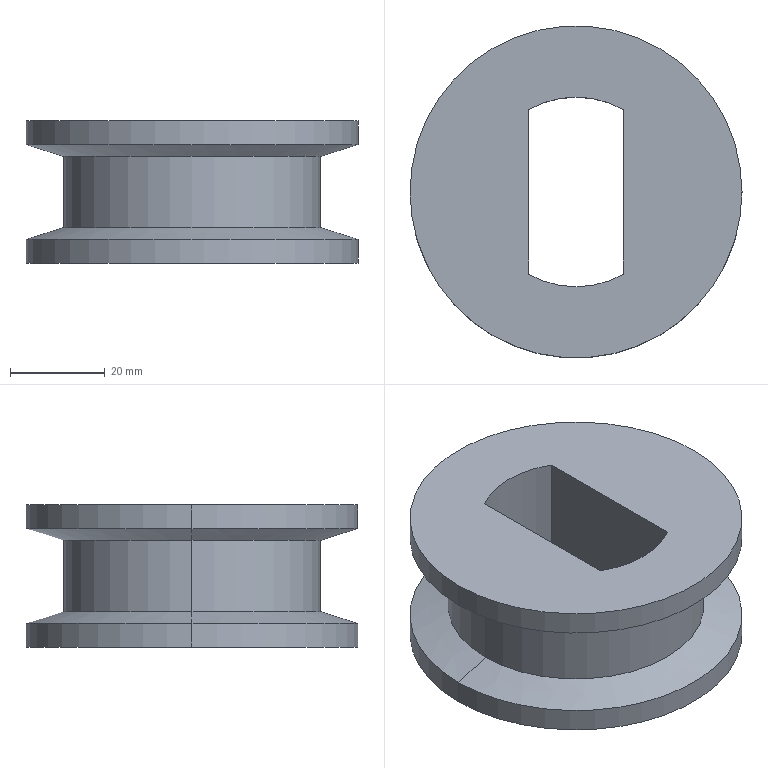Part | SolidWorks | 1 solid | 16 faces | box 70 x 70 x 30 mm | volume 65058 mm3 | cylinder 8 | cone 4 | plane 4 | commonest cylinder face diameters 70 x4 40 x2 54 x2
STEP:
#1=CARTESIAN_POINT('',(-27.,0.,7.5));
#2=VERTEX_POINT('',#1);
#3=CARTESIAN_POINT('',(27.,0.,7.5));
#4=VERTEX_POINT('',#3);
#5=CARTESIAN_POINT('',(0.,0.,7.5));
#6=DIRECTION('',(0.,0.,-1.));
#7=DIRECTION('',(-1.,0.,0.));
#8=AXIS2_PLACEMENT_3D('',#5,#6,#7);
#9=CIRCLE('',#8,27.);
#10=EDGE_CURVE('',#2,#4,#9,.T.);
#11=ORIENTED_EDGE('',*,*,#10,.T.);
#12=CARTESIAN_POINT('',(27.,0.,-7.5));
#13=VERTEX_POINT('',#12);
#14=CARTESIAN_POINT('',(27.,0.,-15.));
#15=DIRECTION('',(0.,0.,-1.));
#16=VECTOR('',#15,1000.);
#17=LINE('',#14,#16);
#18=EDGE_CURVE('',#4,#13,#17,.T.);
#19=ORIENTED_EDGE('',*,*,#18,.T.);
#20=CARTESIAN_POINT('',(-27.,0.,-7.5));
#21=VERTEX_POINT('',#20);
#22=CARTESIAN_POINT('',(0.,0.,-7.5));
#23=DIRECTION('',(0.,0.,-1.));
#24=DIRECTION('',(-1.,0.,0.));
#25=AXIS2_PLACEMENT_3D('',#22,#23,#24);
#26=CIRCLE('',#25,27.);
#27=EDGE_CURVE('',#21,#13,#26,.T.);
#28=ORIENTED_EDGE('',*,*,#27,.F.);
#29=CARTESIAN_POINT('',(-27.,0.,-15.));
#30=DIRECTION('',(0.,0.,-1.));
#31=VECTOR('',#30,1000.);
#32=LINE('',#29,#31);
#33=EDGE_CURVE('',#2,#21,#32,.T.);
#34=ORIENTED_EDGE('',*,*,#33,.F.);
#35=EDGE_LOOP('',(#11,#19,#28,#34));
#36=FACE_OUTER_BOUND('',#35,.T.);
#37=CARTESIAN_POINT('',(0.,0.,-15.));
#38=DIRECTION('',(0.,0.,-1.));
#39=DIRECTION('',(-1.,0.,0.));
#40=AXIS2_PLACEMENT_3D('',#37,#38,#39);
#41=CYLINDRICAL_SURFACE('',#40,27.);
#42=ADVANCED_FACE('',(#36),#41,.T.);
#43=ORIENTED_EDGE('',*,*,#10,.F.);
#44=CARTESIAN_POINT('',(-35.,0.,10.));
#45=VERTEX_POINT('',#44);
#46=CARTESIAN_POINT('',(-35.,0.,10.));
#47=DIRECTION('',(-0.9545,0.,0.2983));
#48=VECTOR('',#47,1000.);
#49=LINE('',#46,#48);
#50=EDGE_CURVE('',#2,#45,#49,.T.);
#51=ORIENTED_EDGE('',*,*,#50,.T.);
#52=CARTESIAN_POINT('',(35.,0.,10.));
#53=VERTEX_POINT('',#52);
#54=CARTESIAN_POINT('',(0.,0.,10.));
#55=DIRECTION('',(0.,0.,-1.));
#56=DIRECTION('',(-1.,0.,0.));
#57=AXIS2_PLACEMENT_3D('',#54,#55,#56);
#58=CIRCLE('',#57,35.);
#59=EDGE_CURVE('',#45,#53,#58,.T.);
#60=ORIENTED_EDGE('',*,*,#59,.T.);
#61=CARTESIAN_POINT('',(35.,0.,10.));
#62=DIRECTION('',(0.9545,0.,0.2983));
#63=VECTOR('',#62,1000.);
#64=LINE('',#61,#63);
#65=EDGE_CURVE('',#4,#53,#64,.T.);
#66=ORIENTED_EDGE('',*,*,#65,.F.);
#67=EDGE_LOOP('',(#43,#51,#60,#66));
#68=FACE_OUTER_BOUND('',#67,.T.);
#69=CARTESIAN_POINT('',(0.,0.,10.));
#70=DIRECTION('',(0.,0.,1.));
#71=DIRECTION('',(1.,0.,0.));
#72=AXIS2_PLACEMENT_3D('',#69,#70,#71);
#73=CONICAL_SURFACE('',#72,35.,1.268);
#74=ADVANCED_FACE('',(#68),#73,.T.);
#75=ORIENTED_EDGE('',*,*,#27,.T.);
#76=CARTESIAN_POINT('',(35.,0.,-10.));
#77=VERTEX_POINT('',#76);
#78=CARTESIAN_POINT('',(27.,0.,-7.5));
#79=DIRECTION('',(0.9545,0.,-0.2983));
#80=VECTOR('',#79,1000.);
#81=LINE('',#78,#80);
#82=EDGE_CURVE('',#13,#77,#81,.T.);
#83=ORIENTED_EDGE('',*,*,#82,.T.);
#84=CARTESIAN_POINT('',(-35.,0.,-10.));
#85=VERTEX_POINT('',#84);
#86=CARTESIAN_POINT('',(0.,0.,-10.));
#87=DIRECTION('',(0.,0.,-1.));
#88=DIRECTION('',(-1.,0.,0.));
#89=AXIS2_PLACEMENT_3D('',#86,#87,#88);
#90=CIRCLE('',#89,35.);
#91=EDGE_CURVE('',#85,#77,#90,.T.);
#92=ORIENTED_EDGE('',*,*,#91,.F.);
#93=CARTESIAN_POINT('',(-27.,0.,-7.5));
#94=DIRECTION('',(-0.9545,0.,-0.2983));
#95=VECTOR('',#94,1000.);
#96=LINE('',#93,#95);
#97=EDGE_CURVE('',#21,#85,#96,.T.);
#98=ORIENTED_EDGE('',*,*,#97,.F.);
#99=EDGE_LOOP('',(#75,#83,#92,#98));
#100=FACE_OUTER_BOUND('',#99,.T.);
#101=CARTESIAN_POINT('',(0.,0.,-7.5));
#102=DIRECTION('',(0.,0.,-1.));
#103=DIRECTION('',(-1.,0.,0.));
#104=AXIS2_PLACEMENT_3D('',#101,#102,#103);
#105=CONICAL_SURFACE('',#104,27.,1.268);
#106=ADVANCED_FACE('',(#100),#105,.T.);
#107=CARTESIAN_POINT('',(35.,0.,15.));
#108=VERTEX_POINT('',#107);
#109=CARTESIAN_POINT('',(-35.,0.,15.));
#110=VERTEX_POINT('',#109);
#111=CARTESIAN_POINT('',(0.,0.,15.));
#112=DIRECTION('',(0.,0.,1.));
#113=DIRECTION('',(1.,0.,0.));
#114=AXIS2_PLACEMENT_3D('',#111,#112,#113);
#115=CIRCLE('',#114,35.);
#116=EDGE_CURVE('',#108,#110,#115,.T.);
#117=ORIENTED_EDGE('',*,*,#116,.F.);
#118=CARTESIAN_POINT('',(35.,0.,15.));
#119=DIRECTION('',(0.,0.,-1.));
#120=VECTOR('',#119,1000.);
#121=LINE('',#118,#120);
#122=EDGE_CURVE('',#108,#53,#121,.T.);
#123=ORIENTED_EDGE('',*,*,#122,.T.);
#124=ORIENTED_EDGE('',*,*,#59,.F.);
#125=CARTESIAN_POINT('',(-35.,0.,15.));
#126=DIRECTION('',(0.,0.,-1.));
#127=VECTOR('',#126,1000.);
#128=LINE('',#125,#127);
#129=EDGE_CURVE('',#110,#45,#128,.T.);
#130=ORIENTED_EDGE('',*,*,#129,.F.);
#131=EDGE_LOOP('',(#117,#123,#124,#130));
#132=FACE_OUTER_BOUND('',#131,.T.);
#133=CARTESIAN_POINT('',(0.,0.,15.));
#134=DIRECTION('',(0.,0.,-1.));
#135=DIRECTION('',(-1.,0.,0.));
#136=AXIS2_PLACEMENT_3D('',#133,#134,#135);
#137=CYLINDRICAL_SURFACE('',#136,35.);
#138=ADVANCED_FACE('',(#132),#137,.T.);
#139=ORIENTED_EDGE('',*,*,#91,.T.);
#140=CARTESIAN_POINT('',(35.,0.,-15.));
#141=VERTEX_POINT('',#140);
#142=CARTESIAN_POINT('',(35.,0.,15.));
#143=DIRECTION('',(0.,0.,-1.));
#144=VECTOR('',#143,1000.);
#145=LINE('',#142,#144);
#146=EDGE_CURVE('',#77,#141,#145,.T.);
#147=ORIENTED_EDGE('',*,*,#146,.T.);
#148=CARTESIAN_POINT('',(-35.,0.,-15.));
#149=VERTEX_POINT('',#148);
#150=CARTESIAN_POINT('',(0.,0.,-15.));
#151=DIRECTION('',(0.,0.,1.));
#152=DIRECTION('',(1.,0.,0.));
#153=AXIS2_PLACEMENT_3D('',#150,#151,#152);
#154=CIRCLE('',#153,35.);
#155=EDGE_CURVE('',#141,#149,#154,.T.);
#156=ORIENTED_EDGE('',*,*,#155,.T.);
#157=CARTESIAN_POINT('',(-35.,0.,15.));
#158=DIRECTION('',(0.,0.,-1.));
#159=VECTOR('',#158,1000.);
#160=LINE('',#157,#159);
#161=EDGE_CURVE('',#85,#149,#160,.T.);
#162=ORIENTED_EDGE('',*,*,#161,.F.);
#163=EDGE_LOOP('',(#139,#147,#156,#162));
#164=FACE_OUTER_BOUND('',#163,.T.);
#165=CARTESIAN_POINT('',(0.,0.,15.));
#166=DIRECTION('',(0.,0.,-1.));
#167=DIRECTION('',(-1.,0.,0.));
#168=AXIS2_PLACEMENT_3D('',#165,#166,#167);
#169=CYLINDRICAL_SURFACE('',#168,35.);
#170=ADVANCED_FACE('',(#164),#169,.T.);
#171=ORIENTED_EDGE('',*,*,#146,.F.);
#172=CARTESIAN_POINT('',(0.,0.,-10.));
#173=DIRECTION('',(0.,0.,-1.));
#174=DIRECTION('',(-1.,0.,0.));
#175=AXIS2_PLACEMENT_3D('',#172,#173,#174);
#176=CIRCLE('',#175,35.);
#177=EDGE_CURVE('',#77,#85,#176,.T.);
#178=ORIENTED_EDGE('',*,*,#177,.T.);
#179=ORIENTED_EDGE('',*,*,#161,.T.);
#180=CARTESIAN_POINT('',(0.,0.,-15.));
#181=DIRECTION('',(0.,0.,1.));
#182=DIRECTION('',(1.,0.,0.));
#183=AXIS2_PLACEMENT_3D('',#180,#181,#182);
#184=CIRCLE('',#183,35.);
#185=EDGE_CURVE('',#149,#141,#184,.T.);
#186=ORIENTED_EDGE('',*,*,#185,.T.);
#187=EDGE_LOOP('',(#171,#178,#179,#186));
#188=FACE_OUTER_BOUND('',#187,.T.);
#189=CARTESIAN_POINT('',(0.,0.,15.));
#190=DIRECTION('',(0.,0.,-1.));
#191=DIRECTION('',(-1.,0.,0.));
#192=AXIS2_PLACEMENT_3D('',#189,#190,#191);
#193=CYLINDRICAL_SURFACE('',#192,35.);
#194=ADVANCED_FACE('',(#188),#193,.T.);
#195=CARTESIAN_POINT('',(10.,17.321,-15.));
#196=VERTEX_POINT('',#195);
#197=CARTESIAN_POINT('',(10.,-17.321,-15.));
#198=VERTEX_POINT('',#197);
#199=CARTESIAN_POINT('',(10.,0.,-15.));
#200=DIRECTION('',(0.,-1.,0.));
#201=VECTOR('',#200,1000.);
#202=LINE('',#199,#201);
#203=EDGE_CURVE('',#196,#198,#202,.T.);
#204=ORIENTED_EDGE('',*,*,#203,.T.);
#205=CARTESIAN_POINT('',(10.,-17.321,15.));
#206=VERTEX_POINT('',#205);
#207=CARTESIAN_POINT('',(10.,-17.321,15.));
#208=DIRECTION('',(0.,0.,-1.));
#209=VECTOR('',#208,1000.);
#210=LINE('',#207,#209);
#211=EDGE_CURVE('',#206,#198,#210,.T.);
#212=ORIENTED_EDGE('',*,*,#211,.F.);
#213=CARTESIAN_POINT('',(10.,17.321,15.));
#214=VERTEX_POINT('',#213);
#215=CARTESIAN_POINT('',(10.,0.,15.));
#216=DIRECTION('',(0.,-1.,0.));
#217=VECTOR('',#216,1000.);
#218=LINE('',#215,#217);
#219=EDGE_CURVE('',#214,#206,#218,.T.);
#220=ORIENTED_EDGE('',*,*,#219,.F.);
#221=CARTESIAN_POINT('',(10.,17.321,15.));
#222=DIRECTION('',(0.,0.,-1.));
#223=VECTOR('',#222,1000.);
#224=LINE('',#221,#223);
#225=EDGE_CURVE('',#214,#196,#224,.T.);
#226=ORIENTED_EDGE('',*,*,#225,.T.);
#227=EDGE_LOOP('',(#204,#212,#220,#226));
#228=FACE_OUTER_BOUND('',#227,.T.);
#229=CARTESIAN_POINT('',(10.,0.,15.));
#230=DIRECTION('',(1.,0.,0.));
#231=DIRECTION('',(0.,0.,-1.));
#232=AXIS2_PLACEMENT_3D('',#229,#230,#231);
#233=PLANE('',#232);
#234=ADVANCED_FACE('',(#228),#233,.F.);
#235=CARTESIAN_POINT('',(-10.,-17.321,-15.));
#236=VERTEX_POINT('',#235);
#237=CARTESIAN_POINT('',(0.,0.,-15.));
#238=DIRECTION('',(0.,0.,1.));
#239=DIRECTION('',(1.,0.,0.));
#240=AXIS2_PLACEMENT_3D('',#237,#238,#239);
#241=CIRCLE('',#240,20.);
#242=EDGE_CURVE('',#236,#198,#241,.T.);
#243=ORIENTED_EDGE('',*,*,#242,.F.);
#244=CARTESIAN_POINT('',(-10.,-17.321,15.));
#245=VERTEX_POINT('',#244);
#246=CARTESIAN_POINT('',(-10.,-17.321,15.));
#247=DIRECTION('',(0.,0.,-1.));
#248=VECTOR('',#247,1000.);
#249=LINE('',#246,#248);
#250=EDGE_CURVE('',#245,#236,#249,.T.);
#251=ORIENTED_EDGE('',*,*,#250,.F.);
#252=CARTESIAN_POINT('',(0.,0.,15.));
#253=DIRECTION('',(0.,0.,1.));
#254=DIRECTION('',(1.,0.,0.));
#255=AXIS2_PLACEMENT_3D('',#252,#253,#254);
#256=CIRCLE('',#255,20.);
#257=EDGE_CURVE('',#245,#206,#256,.T.);
#258=ORIENTED_EDGE('',*,*,#257,.T.);
#259=ORIENTED_EDGE('',*,*,#211,.T.);
#260=EDGE_LOOP('',(#243,#251,#258,#259));
#261=FACE_OUTER_BOUND('',#260,.T.);
#262=CARTESIAN_POINT('',(0.,0.,15.));
#263=DIRECTION('',(0.,0.,-1.));
#264=DIRECTION('',(-1.,0.,0.));
#265=AXIS2_PLACEMENT_3D('',#262,#263,#264);
#266=CYLINDRICAL_SURFACE('',#265,20.);
#267=ADVANCED_FACE('',(#261),#266,.F.);
#268=CARTESIAN_POINT('',(-10.,17.321,-15.));
#269=VERTEX_POINT('',#268);
#270=CARTESIAN_POINT('',(-10.,0.,-15.));
#271=DIRECTION('',(0.,-1.,0.));
#272=VECTOR('',#271,1000.);
#273=LINE('',#270,#272);
#274=EDGE_CURVE('',#269,#236,#273,.T.);
#275=ORIENTED_EDGE('',*,*,#274,.F.);
#276=CARTESIAN_POINT('',(-10.,17.321,15.));
#277=VERTEX_POINT('',#276);
#278=CARTESIAN_POINT('',(-10.,17.321,15.));
#279=DIRECTION('',(0.,0.,-1.));
#280=VECTOR('',#279,1000.);
#281=LINE('',#278,#280);
#282=EDGE_CURVE('',#277,#269,#281,.T.);
#283=ORIENTED_EDGE('',*,*,#282,.F.);
#284=CARTESIAN_POINT('',(-10.,0.,15.));
#285=DIRECTION('',(0.,-1.,0.));
#286=VECTOR('',#285,1000.);
#287=LINE('',#284,#286);
#288=EDGE_CURVE('',#277,#245,#287,.T.);
#289=ORIENTED_EDGE('',*,*,#288,.T.);
#290=ORIENTED_EDGE('',*,*,#250,.T.);
#291=EDGE_LOOP('',(#275,#283,#289,#290));
#292=FACE_OUTER_BOUND('',#291,.T.);
#293=CARTESIAN_POINT('',(-10.,0.,15.));
#294=DIRECTION('',(1.,0.,0.));
#295=DIRECTION('',(0.,0.,-1.));
#296=AXIS2_PLACEMENT_3D('',#293,#294,#295);
#297=PLANE('',#296);
#298=ADVANCED_FACE('',(#292),#297,.T.);
#299=CARTESIAN_POINT('',(0.,0.,-15.));
#300=DIRECTION('',(0.,0.,1.));
#301=DIRECTION('',(1.,0.,0.));
#302=AXIS2_PLACEMENT_3D('',#299,#300,#301);
#303=CIRCLE('',#302,20.);
#304=EDGE_CURVE('',#196,#269,#303,.T.);
#305=ORIENTED_EDGE('',*,*,#304,.F.);
#306=ORIENTED_EDGE('',*,*,#225,.F.);
#307=CARTESIAN_POINT('',(0.,0.,15.));
#308=DIRECTION('',(0.,0.,1.));
#309=DIRECTION('',(1.,0.,0.));
#310=AXIS2_PLACEMENT_3D('',#307,#308,#309);
#311=CIRCLE('',#310,20.);
#312=EDGE_CURVE('',#214,#277,#311,.T.);
#313=ORIENTED_EDGE('',*,*,#312,.T.);
#314=ORIENTED_EDGE('',*,*,#282,.T.);
#315=EDGE_LOOP('',(#305,#306,#313,#314));
#316=FACE_OUTER_BOUND('',#315,.T.);
#317=CARTESIAN_POINT('',(0.,0.,15.));
#318=DIRECTION('',(0.,0.,-1.));
#319=DIRECTION('',(-1.,0.,0.));
#320=AXIS2_PLACEMENT_3D('',#317,#318,#319);
#321=CYLINDRICAL_SURFACE('',#320,20.);
#322=ADVANCED_FACE('',(#316),#321,.F.);
#323=ORIENTED_EDGE('',*,*,#122,.F.);
#324=CARTESIAN_POINT('',(0.,0.,15.));
#325=DIRECTION('',(0.,0.,1.));
#326=DIRECTION('',(1.,0.,0.));
#327=AXIS2_PLACEMENT_3D('',#324,#325,#326);
#328=CIRCLE('',#327,35.);
#329=EDGE_CURVE('',#110,#108,#328,.T.);
#330=ORIENTED_EDGE('',*,*,#329,.F.);
#331=ORIENTED_EDGE('',*,*,#129,.T.);
#332=CARTESIAN_POINT('',(0.,0.,10.));
#333=DIRECTION('',(0.,0.,-1.));
#334=DIRECTION('',(-1.,0.,0.));
#335=AXIS2_PLACEMENT_3D('',#332,#333,#334);
#336=CIRCLE('',#335,35.);
#337=EDGE_CURVE('',#53,#45,#336,.T.);
#338=ORIENTED_EDGE('',*,*,#337,.F.);
#339=EDGE_LOOP('',(#323,#330,#331,#338));
#340=FACE_OUTER_BOUND('',#339,.T.);
#341=CARTESIAN_POINT('',(0.,0.,15.));
#342=DIRECTION('',(0.,0.,-1.));
#343=DIRECTION('',(-1.,0.,0.));
#344=AXIS2_PLACEMENT_3D('',#341,#342,#343);
#345=CYLINDRICAL_SURFACE('',#344,35.);
#346=ADVANCED_FACE('',(#340),#345,.T.);
#347=ORIENTED_EDGE('',*,*,#219,.T.);
#348=ORIENTED_EDGE('',*,*,#257,.F.);
#349=ORIENTED_EDGE('',*,*,#288,.F.);
#350=ORIENTED_EDGE('',*,*,#312,.F.);
#351=EDGE_LOOP('',(#347,#348,#349,#350));
#352=FACE_BOUND('',#351,.T.);
#353=ORIENTED_EDGE('',*,*,#329,.T.);
#354=ORIENTED_EDGE('',*,*,#116,.T.);
#355=EDGE_LOOP('',(#353,#354));
#356=FACE_OUTER_BOUND('',#355,.T.);
#357=CARTESIAN_POINT('',(0.,0.,15.));
#358=DIRECTION('',(0.,0.,1.));
#359=DIRECTION('',(1.,0.,0.));
#360=AXIS2_PLACEMENT_3D('',#357,#358,#359);
#361=PLANE('',#360);
#362=ADVANCED_FACE('',(#352,#356),#361,.T.);
#363=ORIENTED_EDGE('',*,*,#203,.F.);
#364=ORIENTED_EDGE('',*,*,#304,.T.);
#365=ORIENTED_EDGE('',*,*,#274,.T.);
#366=ORIENTED_EDGE('',*,*,#242,.T.);
#367=EDGE_LOOP('',(#363,#364,#365,#366));
#368=FACE_BOUND('',#367,.T.);
#369=ORIENTED_EDGE('',*,*,#185,.F.);
#370=ORIENTED_EDGE('',*,*,#155,.F.);
#371=EDGE_LOOP('',(#369,#370));
#372=FACE_OUTER_BOUND('',#371,.T.);
#373=CARTESIAN_POINT('',(0.,0.,-15.));
#374=DIRECTION('',(0.,0.,1.));
#375=DIRECTION('',(1.,0.,0.));
#376=AXIS2_PLACEMENT_3D('',#373,#374,#375);
#377=PLANE('',#376);
#378=ADVANCED_FACE('',(#368,#372),#377,.F.);
#379=ORIENTED_EDGE('',*,*,#82,.F.);
#380=CARTESIAN_POINT('',(0.,0.,-7.5));
#381=DIRECTION('',(0.,0.,-1.));
#382=DIRECTION('',(-1.,0.,0.));
#383=AXIS2_PLACEMENT_3D('',#380,#381,#382);
#384=CIRCLE('',#383,27.);
#385=EDGE_CURVE('',#13,#21,#384,.T.);
#386=ORIENTED_EDGE('',*,*,#385,.T.);
#387=ORIENTED_EDGE('',*,*,#97,.T.);
#388=ORIENTED_EDGE('',*,*,#177,.F.);
#389=EDGE_LOOP('',(#379,#386,#387,#388));
#390=FACE_OUTER_BOUND('',#389,.T.);
#391=CARTESIAN_POINT('',(0.,0.,-7.5));
#392=DIRECTION('',(0.,0.,-1.));
#393=DIRECTION('',(-1.,0.,0.));
#394=AXIS2_PLACEMENT_3D('',#391,#392,#393);
#395=CONICAL_SURFACE('',#394,27.,1.268);
#396=ADVANCED_FACE('',(#390),#395,.T.);
#397=ORIENTED_EDGE('',*,*,#50,.F.);
#398=CARTESIAN_POINT('',(0.,0.,7.5));
#399=DIRECTION('',(0.,0.,-1.));
#400=DIRECTION('',(-1.,0.,0.));
#401=AXIS2_PLACEMENT_3D('',#398,#399,#400);
#402=CIRCLE('',#401,27.);
#403=EDGE_CURVE('',#4,#2,#402,.T.);
#404=ORIENTED_EDGE('',*,*,#403,.F.);
#405=ORIENTED_EDGE('',*,*,#65,.T.);
#406=ORIENTED_EDGE('',*,*,#337,.T.);
#407=EDGE_LOOP('',(#397,#404,#405,#406));
#408=FACE_OUTER_BOUND('',#407,.T.);
#409=CARTESIAN_POINT('',(0.,0.,10.));
#410=DIRECTION('',(0.,0.,1.));
#411=DIRECTION('',(1.,0.,0.));
#412=AXIS2_PLACEMENT_3D('',#409,#410,#411);
#413=CONICAL_SURFACE('',#412,35.,1.268);
#414=ADVANCED_FACE('',(#408),#413,.T.);
#415=ORIENTED_EDGE('',*,*,#18,.F.);
#416=ORIENTED_EDGE('',*,*,#403,.T.);
#417=ORIENTED_EDGE('',*,*,#33,.T.);
#418=ORIENTED_EDGE('',*,*,#385,.F.);
#419=EDGE_LOOP('',(#415,#416,#417,#418));
#420=FACE_OUTER_BOUND('',#419,.T.);
#421=CARTESIAN_POINT('',(0.,0.,-15.));
#422=DIRECTION('',(0.,0.,-1.));
#423=DIRECTION('',(-1.,0.,0.));
#424=AXIS2_PLACEMENT_3D('',#421,#422,#423);
#425=CYLINDRICAL_SURFACE('',#424,27.);
#426=ADVANCED_FACE('',(#420),#425,.T.);
#427=CLOSED_SHELL('',(#42,#74,#106,#138,#170,#194,#234,#267,#298,#322,#346,#362,#378,#396,#414,#426));
#428=MANIFOLD_SOLID_BREP('',#427);
#429=CARTESIAN_POINT('',(0.,0.,0.));
#430=DIRECTION('',(0.,0.,1.));
#431=DIRECTION('',(1.,0.,0.));
#432=AXIS2_PLACEMENT_3D('',#429,#430,#431);
#433=(LENGTH_UNIT()NAMED_UNIT(*)SI_UNIT(.MILLI.,.METRE.));
#434=UNCERTAINTY_MEASURE_WITH_UNIT(LENGTH_MEASURE(0.00001),#433,'','');
#435=(NAMED_UNIT(*)PLANE_ANGLE_UNIT()SI_UNIT($,.RADIAN.));
#436=(NAMED_UNIT(*)SI_UNIT($,.STERADIAN.)SOLID_ANGLE_UNIT());
#437=(GEOMETRIC_REPRESENTATION_CONTEXT(3)GLOBAL_UNCERTAINTY_ASSIGNED_CONTEXT((#434))GLOBAL_UNIT_ASSIGNED_CONTEXT((#433,#435,#436))REPRESENTATION_CONTEXT('',''));
#438=ADVANCED_BREP_SHAPE_REPRESENTATION('',(#428,#432),#437);